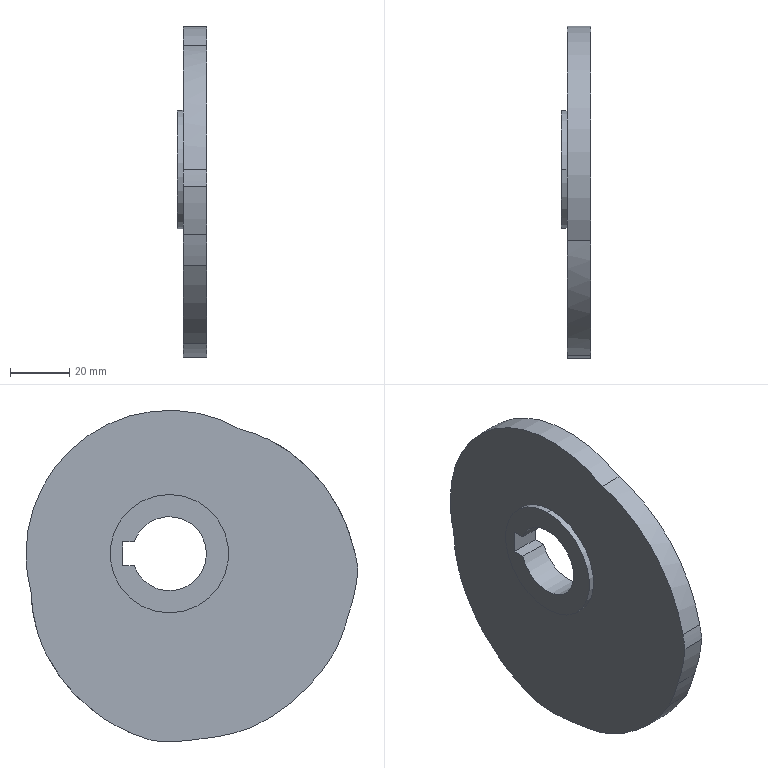Part | NX | 1 solid | 20 faces | box 10 x 112.057 x 111.8 mm | volume 75141 mm3 | cylinder 12 | plane 6 | spline 2 | commonest cylinder face diameters 25 x2 40 x2 96.8 x2 124.139 x1 126.8 x1 127.634 x1
STEP:
#1=CARTESIAN_POINT('',(-4.,46.751,-12.527));
#2=VERTEX_POINT('',#1);
#3=CARTESIAN_POINT('',(-4.,48.4,0.));
#4=VERTEX_POINT('',#3);
#5=CARTESIAN_POINT('',(-4.,0.,0.));
#6=DIRECTION('',(1.,0.,0.));
#7=DIRECTION('',(0.,1.,0.));
#8=AXIS2_PLACEMENT_3D('',#5,#6,#7);
#9=CIRCLE('',#8,48.4);
#10=EDGE_CURVE('',#2,#4,#9,.T.);
#11=ORIENTED_EDGE('',*,*,#10,.F.);
#12=CARTESIAN_POINT('',(-4.,5.526,-63.159));
#13=VERTEX_POINT('',#12);
#14=CARTESIAN_POINT('',(-4.,46.751,-12.527));
#15=CARTESIAN_POINT('',(-4.,46.716,-15.104));
#16=CARTESIAN_POINT('',(-4.,46.362,-18.915));
#17=CARTESIAN_POINT('',(-4.,45.21,-24.184));
#18=CARTESIAN_POINT('',(-4.,44.045,-28.007));
#19=CARTESIAN_POINT('',(-4.,42.505,-31.909));
#20=CARTESIAN_POINT('',(-4.,40.684,-35.618));
#21=CARTESIAN_POINT('',(-4.,38.469,-39.345));
#22=CARTESIAN_POINT('',(-4.,35.998,-42.831));
#23=CARTESIAN_POINT('',(-4.,33.129,-46.264));
#24=CARTESIAN_POINT('',(-4.,30.037,-49.413));
#25=CARTESIAN_POINT('',(-4.,26.555,-52.439));
#26=CARTESIAN_POINT('',(-4.,22.888,-55.142));
#27=CARTESIAN_POINT('',(-4.,18.854,-57.651));
#28=CARTESIAN_POINT('',(-4.,13.277,-60.529));
#29=CARTESIAN_POINT('',(-4.,8.665,-62.261));
#30=CARTESIAN_POINT('',(-4.,5.526,-63.159));
#31=B_SPLINE_CURVE_WITH_KNOTS('',3,(#14,#15,#16,#17,#18,#19,#20,#21,#22,#23,#24,#25,#26,#27,#28,#29,#30),.UNSPECIFIED.,.F.,.F.,(4,1,1,1,1,1,1,1,1,1,1,1,1,1,4),(0.00000001,0.125,0.1875,0.25,0.3125,0.375,0.4375,0.5,0.5625,0.625,0.6875,0.75,0.8125,0.875,1.),.UNSPECIFIED.);
#32=EDGE_CURVE('',#13,#2,#31,.F.);
#33=ORIENTED_EDGE('',*,*,#32,.F.);
#34=CARTESIAN_POINT('',(-4.,-11.009,-62.437));
#35=VERTEX_POINT('',#34);
#36=CARTESIAN_POINT('',(-4.,0.,0.));
#37=DIRECTION('',(1.,0.,0.));
#38=DIRECTION('',(0.,-0.1736,-0.9848));
#39=AXIS2_PLACEMENT_3D('',#36,#37,#38);
#40=CIRCLE('',#39,63.4);
#41=EDGE_CURVE('',#35,#13,#40,.T.);
#42=ORIENTED_EDGE('',*,*,#41,.F.);
#43=CARTESIAN_POINT('',(-4.,-27.428,-58.819));
#44=VERTEX_POINT('',#43);
#45=CARTESIAN_POINT('',(-4.,-5.606,1.151));
#46=DIRECTION('',(1.,0.,0.));
#47=DIRECTION('',(0.,-0.342,-0.9397));
#48=AXIS2_PLACEMENT_3D('',#45,#46,#47);
#49=CIRCLE('',#48,63.817);
#50=EDGE_CURVE('',#44,#35,#49,.T.);
#51=ORIENTED_EDGE('',*,*,#50,.F.);
#52=CARTESIAN_POINT('',(-4.,-56.205,-32.45));
#53=VERTEX_POINT('',#52);
#54=CARTESIAN_POINT('',(-4.,0.,0.));
#55=DIRECTION('',(1.,0.,0.));
#56=DIRECTION('',(0.,-0.866,-0.5));
#57=AXIS2_PLACEMENT_3D('',#54,#55,#56);
#58=CIRCLE('',#57,64.9);
#59=EDGE_CURVE('',#53,#44,#58,.T.);
#60=ORIENTED_EDGE('',*,*,#59,.F.);
#61=CARTESIAN_POINT('',(-4.,-60.047,-21.855));
#62=VERTEX_POINT('',#61);
#63=CARTESIAN_POINT('',(-4.,2.003,-5.352));
#64=DIRECTION('',(1.,0.,0.));
#65=DIRECTION('',(0.,-0.9664,-0.257));
#66=AXIS2_PLACEMENT_3D('',#63,#64,#65);
#67=CIRCLE('',#66,64.207);
#68=EDGE_CURVE('',#62,#53,#67,.T.);
#69=ORIENTED_EDGE('',*,*,#68,.F.);
#70=CARTESIAN_POINT('',(-4.,-63.657,-5.569));
#71=VERTEX_POINT('',#70);
#72=CARTESIAN_POINT('',(-4.,0.,0.));
#73=DIRECTION('',(1.,0.,0.));
#74=DIRECTION('',(0.,-0.9962,-0.08716));
#75=AXIS2_PLACEMENT_3D('',#72,#73,#74);
#76=CIRCLE('',#75,63.9);
#77=EDGE_CURVE('',#71,#62,#76,.T.);
#78=ORIENTED_EDGE('',*,*,#77,.F.);
#79=CARTESIAN_POINT('',(-4.,-62.708,0.000004523));
#80=VERTEX_POINT('',#79);
#81=CARTESIAN_POINT('',(-4.,-2.058,-13.201));
#82=DIRECTION('',(1.,0.,0.));
#83=DIRECTION('',(0.,-0.9771,0.2127));
#84=AXIS2_PLACEMENT_3D('',#81,#82,#83);
#85=CIRCLE('',#84,62.069);
#86=EDGE_CURVE('',#80,#71,#85,.T.);
#87=ORIENTED_EDGE('',*,*,#86,.F.);
#88=CARTESIAN_POINT('',(-4.,-24.2,41.916));
#89=VERTEX_POINT('',#88);
#90=CARTESIAN_POINT('',(-4.,-62.708,0.00001413));
#91=CARTESIAN_POINT('',(-4.,-61.523,5.434));
#92=CARTESIAN_POINT('',(-4.,-57.687,15.802));
#93=CARTESIAN_POINT('',(-4.,-48.504,28.366));
#94=CARTESIAN_POINT('',(-4.,-38.885,35.892));
#95=CARTESIAN_POINT('',(-4.,-30.566,39.982));
#96=CARTESIAN_POINT('',(-4.,-26.354,41.369));
#97=CARTESIAN_POINT('',(-4.,-24.2,41.916));
#98=B_SPLINE_CURVE_WITH_KNOTS('',3,(#90,#91,#92,#93,#94,#95,#96,#97),.UNSPECIFIED.,.F.,.F.,(4,1,1,1,1,4),(0.,0.25,0.5,0.75,0.875,1.),.UNSPECIFIED.);
#99=EDGE_CURVE('',#89,#80,#98,.F.);
#100=ORIENTED_EDGE('',*,*,#99,.F.);
#101=CARTESIAN_POINT('',(-4.,0.,0.));
#102=DIRECTION('',(1.,0.,0.));
#103=DIRECTION('',(0.,1.,0.));
#104=AXIS2_PLACEMENT_3D('',#101,#102,#103);
#105=CIRCLE('',#104,48.4);
#106=EDGE_CURVE('',#4,#89,#105,.T.);
#107=ORIENTED_EDGE('',*,*,#106,.F.);
#108=EDGE_LOOP('',(#11,#33,#42,#51,#60,#69,#78,#87,#100,#107));
#109=FACE_BOUND('',#108,.T.);
#110=CARTESIAN_POINT('',(-4.,0.,20.));
#111=VERTEX_POINT('',#110);
#112=CARTESIAN_POINT('',(-4.,0.,-20.));
#113=VERTEX_POINT('',#112);
#114=CARTESIAN_POINT('',(-4.,0.,0.));
#115=DIRECTION('',(-1.,0.,0.));
#116=DIRECTION('',(0.,0.,1.));
#117=AXIS2_PLACEMENT_3D('',#114,#115,#116);
#118=CIRCLE('',#117,20.);
#119=EDGE_CURVE('',#111,#113,#118,.T.);
#120=ORIENTED_EDGE('',*,*,#119,.F.);
#121=CARTESIAN_POINT('',(-4.,0.,0.));
#122=DIRECTION('',(-1.,0.,0.));
#123=DIRECTION('',(0.,0.,1.));
#124=AXIS2_PLACEMENT_3D('',#121,#122,#123);
#125=CIRCLE('',#124,20.);
#126=EDGE_CURVE('',#113,#111,#125,.T.);
#127=ORIENTED_EDGE('',*,*,#126,.F.);
#128=EDGE_LOOP('',(#120,#127));
#129=FACE_BOUND('',#128,.T.);
#130=CARTESIAN_POINT('',(-4.,0.,0.));
#131=DIRECTION('',(1.,0.,0.));
#132=DIRECTION('',(0.,1.,0.));
#133=AXIS2_PLACEMENT_3D('',#130,#131,#132);
#134=PLANE('',#133);
#135=ADVANCED_FACE('',(#109,#129),#134,.F.);
#136=CARTESIAN_POINT('',(4.,48.4,0.));
#137=VERTEX_POINT('',#136);
#138=CARTESIAN_POINT('',(-4.,48.4,0.));
#139=DIRECTION('',(1.,0.,0.));
#140=VECTOR('',#139,1000.);
#141=LINE('',#138,#140);
#142=EDGE_CURVE('',#4,#137,#141,.T.);
#143=ORIENTED_EDGE('',*,*,#142,.F.);
#144=ORIENTED_EDGE('',*,*,#106,.T.);
#145=CARTESIAN_POINT('',(4.,-24.2,41.916));
#146=VERTEX_POINT('',#145);
#147=CARTESIAN_POINT('',(-4.,-24.2,41.916));
#148=CARTESIAN_POINT('',(-1.333,-24.2,41.916));
#149=CARTESIAN_POINT('',(1.333,-24.2,41.916));
#150=CARTESIAN_POINT('',(4.,-24.2,41.916));
#151=B_SPLINE_CURVE_WITH_KNOTS('',3,(#147,#148,#149,#150),.UNSPECIFIED.,.F.,.F.,(4,4),(0.,1.),.UNSPECIFIED.);
#152=EDGE_CURVE('',#89,#146,#151,.T.);
#153=ORIENTED_EDGE('',*,*,#152,.T.);
#154=CARTESIAN_POINT('',(4.,0.,0.));
#155=DIRECTION('',(-1.,0.,0.));
#156=DIRECTION('',(0.,-0.5,0.866));
#157=AXIS2_PLACEMENT_3D('',#154,#155,#156);
#158=CIRCLE('',#157,48.4);
#159=EDGE_CURVE('',#146,#137,#158,.T.);
#160=ORIENTED_EDGE('',*,*,#159,.T.);
#161=EDGE_LOOP('',(#143,#144,#153,#160));
#162=FACE_BOUND('',#161,.T.);
#163=CARTESIAN_POINT('',(-4.,0.,0.));
#164=DIRECTION('',(1.,0.,0.));
#165=DIRECTION('',(0.,1.,0.));
#166=AXIS2_PLACEMENT_3D('',#163,#164,#165);
#167=CYLINDRICAL_SURFACE('',#166,48.4);
#168=ADVANCED_FACE('',(#162),#167,.T.);
#169=CARTESIAN_POINT('',(4.,5.526,-63.159));
#170=VERTEX_POINT('',#169);
#171=CARTESIAN_POINT('',(-4.,5.526,-63.159));
#172=CARTESIAN_POINT('',(-1.333,5.526,-63.159));
#173=CARTESIAN_POINT('',(1.333,5.526,-63.159));
#174=CARTESIAN_POINT('',(4.,5.526,-63.159));
#175=B_SPLINE_CURVE_WITH_KNOTS('',3,(#171,#172,#173,#174),.UNSPECIFIED.,.F.,.F.,(4,4),(0.,1.),.UNSPECIFIED.);
#176=EDGE_CURVE('',#13,#170,#175,.T.);
#177=ORIENTED_EDGE('',*,*,#176,.F.);
#178=ORIENTED_EDGE('',*,*,#32,.T.);
#179=CARTESIAN_POINT('',(4.,46.751,-12.527));
#180=VERTEX_POINT('',#179);
#181=CARTESIAN_POINT('',(4.,46.751,-12.527));
#182=CARTESIAN_POINT('',(1.333,46.751,-12.527));
#183=CARTESIAN_POINT('',(-1.333,46.751,-12.527));
#184=CARTESIAN_POINT('',(-4.,46.751,-12.527));
#185=B_SPLINE_CURVE_WITH_KNOTS('',3,(#181,#182,#183,#184),.UNSPECIFIED.,.F.,.F.,(4,4),(0.,1.),.UNSPECIFIED.);
#186=EDGE_CURVE('',#180,#2,#185,.T.);
#187=ORIENTED_EDGE('',*,*,#186,.F.);
#188=CARTESIAN_POINT('',(4.,5.526,-63.159));
#189=CARTESIAN_POINT('',(4.,8.665,-62.261));
#190=CARTESIAN_POINT('',(4.,13.278,-60.528));
#191=CARTESIAN_POINT('',(4.,18.853,-57.651));
#192=CARTESIAN_POINT('',(4.,22.889,-55.141));
#193=CARTESIAN_POINT('',(4.,26.554,-52.439));
#194=CARTESIAN_POINT('',(4.,30.038,-49.413));
#195=CARTESIAN_POINT('',(4.,33.129,-46.265));
#196=CARTESIAN_POINT('',(4.,35.998,-42.83));
#197=CARTESIAN_POINT('',(4.,38.468,-39.346));
#198=CARTESIAN_POINT('',(4.,40.684,-35.618));
#199=CARTESIAN_POINT('',(4.,42.505,-31.91));
#200=CARTESIAN_POINT('',(4.,44.046,-28.006));
#201=CARTESIAN_POINT('',(4.,45.21,-24.185));
#202=CARTESIAN_POINT('',(4.,46.362,-18.914));
#203=CARTESIAN_POINT('',(4.,46.716,-15.104));
#204=CARTESIAN_POINT('',(4.,46.751,-12.527));
#205=B_SPLINE_CURVE_WITH_KNOTS('',3,(#188,#189,#190,#191,#192,#193,#194,#195,#196,#197,#198,#199,#200,#201,#202,#203,#204),.UNSPECIFIED.,.F.,.F.,(4,1,1,1,1,1,1,1,1,1,1,1,1,1,4),(0.,0.125,0.1875,0.25,0.3125,0.375,0.4375,0.5,0.5625,0.625,0.6875,0.75,0.8125,0.875,1.),.UNSPECIFIED.);
#206=EDGE_CURVE('',#180,#170,#205,.F.);
#207=ORIENTED_EDGE('',*,*,#206,.T.);
#208=EDGE_LOOP('',(#177,#178,#187,#207));
#209=FACE_BOUND('',#208,.T.);
#210=CARTESIAN_POINT('',(4.,5.526,-63.159));
#211=CARTESIAN_POINT('',(-4.,5.526,-63.159));
#212=CARTESIAN_POINT('',(4.,11.847,-61.351));
#213=CARTESIAN_POINT('',(-4.,11.847,-61.351));
#214=CARTESIAN_POINT('',(4.,23.543,-55.825));
#215=CARTESIAN_POINT('',(-4.,23.543,-55.825));
#216=CARTESIAN_POINT('',(4.,36.792,-43.244));
#217=CARTESIAN_POINT('',(-4.,36.792,-43.244));
#218=CARTESIAN_POINT('',(4.,44.88,-28.132));
#219=CARTESIAN_POINT('',(-4.,44.88,-28.132));
#220=CARTESIAN_POINT('',(4.,46.683,-17.61));
#221=CARTESIAN_POINT('',(-4.,46.683,-17.61));
#222=CARTESIAN_POINT('',(4.,46.751,-12.527));
#223=CARTESIAN_POINT('',(-4.,46.751,-12.527));
#224=B_SPLINE_SURFACE_WITH_KNOTS('',3,1,((#210,#211),(#212,#213),(#214,#215),(#216,#217),(#218,#219),(#220,#221),(#222,#223)),.SURF_OF_LINEAR_EXTRUSION.,.F.,.F.,.F.,(4,1,1,1,4),(2,2),(0.008679,0.2537,0.4987,0.7438,0.9888),(0.,1.),.UNSPECIFIED.);
#225=ADVANCED_FACE('',(#209),#224,.F.);
#226=CARTESIAN_POINT('',(4.,-11.009,-62.437));
#227=VERTEX_POINT('',#226);
#228=CARTESIAN_POINT('',(4.,-11.009,-62.437));
#229=CARTESIAN_POINT('',(1.333,-11.009,-62.437));
#230=CARTESIAN_POINT('',(-1.333,-11.009,-62.437));
#231=CARTESIAN_POINT('',(-4.,-11.009,-62.437));
#232=B_SPLINE_CURVE_WITH_KNOTS('',3,(#228,#229,#230,#231),.UNSPECIFIED.,.F.,.F.,(4,4),(0.,1.),.UNSPECIFIED.);
#233=EDGE_CURVE('',#35,#227,#232,.F.);
#234=ORIENTED_EDGE('',*,*,#233,.F.);
#235=ORIENTED_EDGE('',*,*,#41,.T.);
#236=ORIENTED_EDGE('',*,*,#176,.T.);
#237=CARTESIAN_POINT('',(4.,0.,0.));
#238=DIRECTION('',(-1.,0.,0.));
#239=DIRECTION('',(0.,0.08716,-0.9962));
#240=AXIS2_PLACEMENT_3D('',#237,#238,#239);
#241=CIRCLE('',#240,63.4);
#242=EDGE_CURVE('',#170,#227,#241,.T.);
#243=ORIENTED_EDGE('',*,*,#242,.T.);
#244=EDGE_LOOP('',(#234,#235,#236,#243));
#245=FACE_BOUND('',#244,.T.);
#246=CARTESIAN_POINT('',(-4.,0.,0.));
#247=DIRECTION('',(1.,0.,0.));
#248=DIRECTION('',(0.,-0.1736,-0.9848));
#249=AXIS2_PLACEMENT_3D('',#246,#247,#248);
#250=CYLINDRICAL_SURFACE('',#249,63.4);
#251=ADVANCED_FACE('',(#245),#250,.T.);
#252=CARTESIAN_POINT('',(4.,-27.428,-58.819));
#253=VERTEX_POINT('',#252);
#254=CARTESIAN_POINT('',(4.,-27.428,-58.819));
#255=CARTESIAN_POINT('',(1.333,-27.428,-58.819));
#256=CARTESIAN_POINT('',(-1.333,-27.428,-58.819));
#257=CARTESIAN_POINT('',(-4.,-27.428,-58.819));
#258=B_SPLINE_CURVE_WITH_KNOTS('',3,(#254,#255,#256,#257),.UNSPECIFIED.,.F.,.F.,(4,4),(0.,1.),.UNSPECIFIED.);
#259=EDGE_CURVE('',#253,#44,#258,.T.);
#260=ORIENTED_EDGE('',*,*,#259,.T.);
#261=ORIENTED_EDGE('',*,*,#50,.T.);
#262=ORIENTED_EDGE('',*,*,#233,.T.);
#263=CARTESIAN_POINT('',(4.,-5.606,1.151));
#264=DIRECTION('',(-1.,0.,0.));
#265=DIRECTION('',(0.,-0.08467,-0.9964));
#266=AXIS2_PLACEMENT_3D('',#263,#264,#265);
#267=CIRCLE('',#266,63.817);
#268=EDGE_CURVE('',#227,#253,#267,.T.);
#269=ORIENTED_EDGE('',*,*,#268,.T.);
#270=EDGE_LOOP('',(#260,#261,#262,#269));
#271=FACE_BOUND('',#270,.T.);
#272=CARTESIAN_POINT('',(0.,-5.606,1.151));
#273=DIRECTION('',(-1.,0.,0.));
#274=DIRECTION('',(0.,-0.3419,-0.9397));
#275=AXIS2_PLACEMENT_3D('',#272,#273,#274);
#276=CYLINDRICAL_SURFACE('',#275,63.817);
#277=ADVANCED_FACE('',(#271),#276,.T.);
#278=CARTESIAN_POINT('',(4.,-56.205,-32.45));
#279=VERTEX_POINT('',#278);
#280=CARTESIAN_POINT('',(4.,-56.205,-32.45));
#281=CARTESIAN_POINT('',(1.333,-56.205,-32.45));
#282=CARTESIAN_POINT('',(-1.333,-56.205,-32.45));
#283=CARTESIAN_POINT('',(-4.,-56.205,-32.45));
#284=B_SPLINE_CURVE_WITH_KNOTS('',3,(#280,#281,#282,#283),.UNSPECIFIED.,.F.,.F.,(4,4),(0.,1.),.UNSPECIFIED.);
#285=EDGE_CURVE('',#53,#279,#284,.F.);
#286=ORIENTED_EDGE('',*,*,#285,.F.);
#287=ORIENTED_EDGE('',*,*,#59,.T.);
#288=ORIENTED_EDGE('',*,*,#259,.F.);
#289=CARTESIAN_POINT('',(4.,0.,0.));
#290=DIRECTION('',(-1.,0.,0.));
#291=DIRECTION('',(0.,-0.4227,-0.9063));
#292=AXIS2_PLACEMENT_3D('',#289,#290,#291);
#293=CIRCLE('',#292,64.9);
#294=EDGE_CURVE('',#253,#279,#293,.T.);
#295=ORIENTED_EDGE('',*,*,#294,.T.);
#296=EDGE_LOOP('',(#286,#287,#288,#295));
#297=FACE_BOUND('',#296,.T.);
#298=CARTESIAN_POINT('',(-4.,0.,0.));
#299=DIRECTION('',(1.,0.,0.));
#300=DIRECTION('',(0.,-0.866,-0.5));
#301=AXIS2_PLACEMENT_3D('',#298,#299,#300);
#302=CYLINDRICAL_SURFACE('',#301,64.9);
#303=ADVANCED_FACE('',(#297),#302,.T.);
#304=CARTESIAN_POINT('',(4.,-60.047,-21.855));
#305=VERTEX_POINT('',#304);
#306=CARTESIAN_POINT('',(4.,-60.047,-21.855));
#307=CARTESIAN_POINT('',(1.333,-60.047,-21.855));
#308=CARTESIAN_POINT('',(-1.333,-60.047,-21.855));
#309=CARTESIAN_POINT('',(-4.,-60.047,-21.855));
#310=B_SPLINE_CURVE_WITH_KNOTS('',3,(#306,#307,#308,#309),.UNSPECIFIED.,.F.,.F.,(4,4),(0.,1.),.UNSPECIFIED.);
#311=EDGE_CURVE('',#305,#62,#310,.T.);
#312=ORIENTED_EDGE('',*,*,#311,.T.);
#313=ORIENTED_EDGE('',*,*,#68,.T.);
#314=ORIENTED_EDGE('',*,*,#285,.T.);
#315=CARTESIAN_POINT('',(4.,2.003,-5.352));
#316=DIRECTION('',(-1.,0.,0.));
#317=DIRECTION('',(0.,-0.9066,-0.422));
#318=AXIS2_PLACEMENT_3D('',#315,#316,#317);
#319=CIRCLE('',#318,64.207);
#320=EDGE_CURVE('',#279,#305,#319,.T.);
#321=ORIENTED_EDGE('',*,*,#320,.T.);
#322=EDGE_LOOP('',(#312,#313,#314,#321));
#323=FACE_BOUND('',#322,.T.);
#324=CARTESIAN_POINT('',(0.,2.003,-5.352));
#325=DIRECTION('',(-1.,0.,0.));
#326=DIRECTION('',(0.,-0.9664,-0.257));
#327=AXIS2_PLACEMENT_3D('',#324,#325,#326);
#328=CYLINDRICAL_SURFACE('',#327,64.207);
#329=ADVANCED_FACE('',(#323),#328,.T.);
#330=CARTESIAN_POINT('',(4.,-63.657,-5.569));
#331=VERTEX_POINT('',#330);
#332=CARTESIAN_POINT('',(4.,-63.657,-5.569));
#333=CARTESIAN_POINT('',(1.333,-63.657,-5.569));
#334=CARTESIAN_POINT('',(-1.333,-63.657,-5.569));
#335=CARTESIAN_POINT('',(-4.,-63.657,-5.569));
#336=B_SPLINE_CURVE_WITH_KNOTS('',3,(#332,#333,#334,#335),.UNSPECIFIED.,.F.,.F.,(4,4),(0.,1.),.UNSPECIFIED.);
#337=EDGE_CURVE('',#71,#331,#336,.F.);
#338=ORIENTED_EDGE('',*,*,#337,.F.);
#339=ORIENTED_EDGE('',*,*,#77,.T.);
#340=ORIENTED_EDGE('',*,*,#311,.F.);
#341=CARTESIAN_POINT('',(4.,0.,0.));
#342=DIRECTION('',(-1.,0.,0.));
#343=DIRECTION('',(0.,-0.9397,-0.342));
#344=AXIS2_PLACEMENT_3D('',#341,#342,#343);
#345=CIRCLE('',#344,63.9);
#346=EDGE_CURVE('',#305,#331,#345,.T.);
#347=ORIENTED_EDGE('',*,*,#346,.T.);
#348=EDGE_LOOP('',(#338,#339,#340,#347));
#349=FACE_BOUND('',#348,.T.);
#350=CARTESIAN_POINT('',(-4.,0.,0.));
#351=DIRECTION('',(1.,0.,0.));
#352=DIRECTION('',(0.,-0.9962,-0.08716));
#353=AXIS2_PLACEMENT_3D('',#350,#351,#352);
#354=CYLINDRICAL_SURFACE('',#353,63.9);
#355=ADVANCED_FACE('',(#349),#354,.T.);
#356=CARTESIAN_POINT('',(4.,-62.708,0.000004523));
#357=VERTEX_POINT('',#356);
#358=CARTESIAN_POINT('',(4.,-62.708,0.00001413));
#359=CARTESIAN_POINT('',(1.333,-62.708,0.00001413));
#360=CARTESIAN_POINT('',(-1.333,-62.708,0.00001413));
#361=CARTESIAN_POINT('',(-4.,-62.708,0.00001413));
#362=B_SPLINE_CURVE_WITH_KNOTS('',3,(#358,#359,#360,#361),.UNSPECIFIED.,.F.,.F.,(4,4),(0.,1.),.UNSPECIFIED.);
#363=EDGE_CURVE('',#357,#80,#362,.T.);
#364=ORIENTED_EDGE('',*,*,#363,.T.);
#365=ORIENTED_EDGE('',*,*,#86,.T.);
#366=ORIENTED_EDGE('',*,*,#337,.T.);
#367=CARTESIAN_POINT('',(4.,-2.058,-13.201));
#368=DIRECTION('',(-1.,0.,0.));
#369=DIRECTION('',(0.,-0.9924,0.123));
#370=AXIS2_PLACEMENT_3D('',#367,#368,#369);
#371=CIRCLE('',#370,62.069);
#372=EDGE_CURVE('',#331,#357,#371,.T.);
#373=ORIENTED_EDGE('',*,*,#372,.T.);
#374=EDGE_LOOP('',(#364,#365,#366,#373));
#375=FACE_BOUND('',#374,.T.);
#376=CARTESIAN_POINT('',(0.,-2.058,-13.201));
#377=DIRECTION('',(-1.,0.,0.));
#378=DIRECTION('',(0.,-0.9771,0.2127));
#379=AXIS2_PLACEMENT_3D('',#376,#377,#378);
#380=CYLINDRICAL_SURFACE('',#379,62.069);
#381=ADVANCED_FACE('',(#375),#380,.T.);
#382=ORIENTED_EDGE('',*,*,#152,.F.);
#383=ORIENTED_EDGE('',*,*,#99,.T.);
#384=ORIENTED_EDGE('',*,*,#363,.F.);
#385=CARTESIAN_POINT('',(4.,-24.2,41.916));
#386=CARTESIAN_POINT('',(4.,-26.354,41.369));
#387=CARTESIAN_POINT('',(4.,-30.566,39.981));
#388=CARTESIAN_POINT('',(4.,-38.885,35.892));
#389=CARTESIAN_POINT('',(4.,-48.504,28.366));
#390=CARTESIAN_POINT('',(4.,-57.688,15.802));
#391=CARTESIAN_POINT('',(4.,-61.523,5.435));
#392=CARTESIAN_POINT('',(4.,-62.708,0.00001413));
#393=B_SPLINE_CURVE_WITH_KNOTS('',3,(#385,#386,#387,#388,#389,#390,#391,#392),.UNSPECIFIED.,.F.,.F.,(4,1,1,1,1,4),(0.000000006,0.125,0.25,0.5,0.75,1.),.UNSPECIFIED.);
#394=EDGE_CURVE('',#357,#146,#393,.F.);
#395=ORIENTED_EDGE('',*,*,#394,.T.);
#396=EDGE_LOOP('',(#382,#383,#384,#395));
#397=FACE_BOUND('',#396,.T.);
#398=CARTESIAN_POINT('',(4.,-24.2,41.916));
#399=CARTESIAN_POINT('',(-4.,-24.2,41.916));
#400=CARTESIAN_POINT('',(4.,-32.708,39.757));
#401=CARTESIAN_POINT('',(-4.,-32.708,39.757));
#402=CARTESIAN_POINT('',(4.,-49.707,30.203));
#403=CARTESIAN_POINT('',(-4.,-49.707,30.203));
#404=CARTESIAN_POINT('',(4.,-60.323,10.944));
#405=CARTESIAN_POINT('',(-4.,-60.323,10.944));
#406=CARTESIAN_POINT('',(4.,-62.708,-0.000005119));
#407=CARTESIAN_POINT('',(-4.,-62.708,-0.000005119));
#408=B_SPLINE_SURFACE_WITH_KNOTS('',3,1,((#398,#399),(#400,#401),(#402,#403),(#404,#405),(#406,#407)),.SURF_OF_LINEAR_EXTRUSION.,.F.,.F.,.F.,(4,1,4),(2,2),(0.01117,0.5012,0.9913),(0.,1.),.UNSPECIFIED.);
#409=ADVANCED_FACE('',(#397),#408,.F.);
#410=ORIENTED_EDGE('',*,*,#159,.F.);
#411=ORIENTED_EDGE('',*,*,#394,.F.);
#412=ORIENTED_EDGE('',*,*,#372,.F.);
#413=ORIENTED_EDGE('',*,*,#346,.F.);
#414=ORIENTED_EDGE('',*,*,#320,.F.);
#415=ORIENTED_EDGE('',*,*,#294,.F.);
#416=ORIENTED_EDGE('',*,*,#268,.F.);
#417=ORIENTED_EDGE('',*,*,#242,.F.);
#418=ORIENTED_EDGE('',*,*,#206,.F.);
#419=CARTESIAN_POINT('',(4.,0.,0.));
#420=DIRECTION('',(-1.,0.,0.));
#421=DIRECTION('',(0.,-0.5,0.866));
#422=AXIS2_PLACEMENT_3D('',#419,#420,#421);
#423=CIRCLE('',#422,48.4);
#424=EDGE_CURVE('',#137,#180,#423,.T.);
#425=ORIENTED_EDGE('',*,*,#424,.F.);
#426=EDGE_LOOP('',(#410,#411,#412,#413,#414,#415,#416,#417,#418,#425));
#427=FACE_BOUND('',#426,.T.);
#428=CARTESIAN_POINT('',(4.,11.843,4.));
#429=VERTEX_POINT('',#428);
#430=CARTESIAN_POINT('',(4.,-12.5,0.));
#431=VERTEX_POINT('',#430);
#432=CARTESIAN_POINT('',(4.,0.,0.));
#433=DIRECTION('',(1.,0.,0.));
#434=DIRECTION('',(0.,-1.,0.));
#435=AXIS2_PLACEMENT_3D('',#432,#433,#434);
#436=CIRCLE('',#435,12.5);
#437=EDGE_CURVE('',#429,#431,#436,.T.);
#438=ORIENTED_EDGE('',*,*,#437,.F.);
#439=CARTESIAN_POINT('',(4.,15.8,4.));
#440=VERTEX_POINT('',#439);
#441=CARTESIAN_POINT('',(4.,11.843,4.));
#442=DIRECTION('',(0.,1.,0.));
#443=VECTOR('',#442,1000.);
#444=LINE('',#441,#443);
#445=EDGE_CURVE('',#429,#440,#444,.T.);
#446=ORIENTED_EDGE('',*,*,#445,.T.);
#447=CARTESIAN_POINT('',(4.,15.8,-4.));
#448=VERTEX_POINT('',#447);
#449=CARTESIAN_POINT('',(4.,15.8,4.));
#450=DIRECTION('',(0.,0.,-1.));
#451=VECTOR('',#450,1000.);
#452=LINE('',#449,#451);
#453=EDGE_CURVE('',#440,#448,#452,.T.);
#454=ORIENTED_EDGE('',*,*,#453,.T.);
#455=CARTESIAN_POINT('',(4.,11.843,-4.));
#456=VERTEX_POINT('',#455);
#457=CARTESIAN_POINT('',(4.,15.8,-4.));
#458=DIRECTION('',(0.,-1.,0.));
#459=VECTOR('',#458,1000.);
#460=LINE('',#457,#459);
#461=EDGE_CURVE('',#448,#456,#460,.T.);
#462=ORIENTED_EDGE('',*,*,#461,.T.);
#463=CARTESIAN_POINT('',(4.,0.,0.));
#464=DIRECTION('',(1.,0.,0.));
#465=DIRECTION('',(0.,-1.,0.));
#466=AXIS2_PLACEMENT_3D('',#463,#464,#465);
#467=CIRCLE('',#466,12.5);
#468=EDGE_CURVE('',#431,#456,#467,.T.);
#469=ORIENTED_EDGE('',*,*,#468,.F.);
#470=EDGE_LOOP('',(#438,#446,#454,#462,#469));
#471=FACE_BOUND('',#470,.T.);
#472=CARTESIAN_POINT('',(4.,0.,0.));
#473=DIRECTION('',(1.,0.,0.));
#474=DIRECTION('',(0.,1.,0.));
#475=AXIS2_PLACEMENT_3D('',#472,#473,#474);
#476=PLANE('',#475);
#477=ADVANCED_FACE('',(#427,#471),#476,.T.);
#478=CARTESIAN_POINT('',(-6.,-12.5,0.));
#479=VERTEX_POINT('',#478);
#480=CARTESIAN_POINT('',(-4.4,-12.5,0.));
#481=DIRECTION('',(1.,0.,0.));
#482=VECTOR('',#481,1000.);
#483=LINE('',#480,#482);
#484=EDGE_CURVE('',#479,#431,#483,.T.);
#485=ORIENTED_EDGE('',*,*,#484,.F.);
#486=CARTESIAN_POINT('',(-6.,11.843,4.));
#487=VERTEX_POINT('',#486);
#488=CARTESIAN_POINT('',(-6.,0.,0.));
#489=DIRECTION('',(-1.,0.,0.));
#490=DIRECTION('',(0.,0.9474,-0.32));
#491=AXIS2_PLACEMENT_3D('',#488,#489,#490);
#492=CIRCLE('',#491,12.5);
#493=EDGE_CURVE('',#479,#487,#492,.T.);
#494=ORIENTED_EDGE('',*,*,#493,.T.);
#495=CARTESIAN_POINT('',(4.,11.843,4.));
#496=DIRECTION('',(-1.,0.,0.));
#497=VECTOR('',#496,1000.);
#498=LINE('',#495,#497);
#499=EDGE_CURVE('',#429,#487,#498,.T.);
#500=ORIENTED_EDGE('',*,*,#499,.F.);
#501=ORIENTED_EDGE('',*,*,#437,.T.);
#502=EDGE_LOOP('',(#485,#494,#500,#501));
#503=FACE_BOUND('',#502,.T.);
#504=CARTESIAN_POINT('',(-4.4,0.,0.));
#505=DIRECTION('',(1.,0.,0.));
#506=DIRECTION('',(0.,-1.,0.));
#507=AXIS2_PLACEMENT_3D('',#504,#505,#506);
#508=CYLINDRICAL_SURFACE('',#507,12.5);
#509=ADVANCED_FACE('',(#503),#508,.F.);
#510=CARTESIAN_POINT('',(-6.,15.8,4.));
#511=VERTEX_POINT('',#510);
#512=CARTESIAN_POINT('',(-6.,15.8,4.));
#513=DIRECTION('',(1.,0.,0.));
#514=VECTOR('',#513,1000.);
#515=LINE('',#512,#514);
#516=EDGE_CURVE('',#511,#440,#515,.T.);
#517=ORIENTED_EDGE('',*,*,#516,.T.);
#518=ORIENTED_EDGE('',*,*,#445,.F.);
#519=ORIENTED_EDGE('',*,*,#499,.T.);
#520=CARTESIAN_POINT('',(-6.,11.843,4.));
#521=DIRECTION('',(0.,1.,0.));
#522=VECTOR('',#521,1000.);
#523=LINE('',#520,#522);
#524=EDGE_CURVE('',#487,#511,#523,.T.);
#525=ORIENTED_EDGE('',*,*,#524,.T.);
#526=EDGE_LOOP('',(#517,#518,#519,#525));
#527=FACE_BOUND('',#526,.T.);
#528=CARTESIAN_POINT('',(4.,15.8,4.));
#529=DIRECTION('',(0.,0.,1.));
#530=DIRECTION('',(1.,0.,0.));
#531=AXIS2_PLACEMENT_3D('',#528,#529,#530);
#532=PLANE('',#531);
#533=ADVANCED_FACE('',(#527),#532,.F.);
#534=CARTESIAN_POINT('',(-6.,15.8,-4.));
#535=VERTEX_POINT('',#534);
#536=CARTESIAN_POINT('',(-6.,15.8,-4.));
#537=DIRECTION('',(1.,0.,0.));
#538=VECTOR('',#537,1000.);
#539=LINE('',#536,#538);
#540=EDGE_CURVE('',#535,#448,#539,.T.);
#541=ORIENTED_EDGE('',*,*,#540,.T.);
#542=ORIENTED_EDGE('',*,*,#453,.F.);
#543=ORIENTED_EDGE('',*,*,#516,.F.);
#544=CARTESIAN_POINT('',(-6.,15.8,4.));
#545=DIRECTION('',(0.,0.,-1.));
#546=VECTOR('',#545,1000.);
#547=LINE('',#544,#546);
#548=EDGE_CURVE('',#511,#535,#547,.T.);
#549=ORIENTED_EDGE('',*,*,#548,.T.);
#550=EDGE_LOOP('',(#541,#542,#543,#549));
#551=FACE_BOUND('',#550,.T.);
#552=CARTESIAN_POINT('',(4.,15.8,-4.));
#553=DIRECTION('',(0.,1.,0.));
#554=DIRECTION('',(1.,0.,0.));
#555=AXIS2_PLACEMENT_3D('',#552,#553,#554);
#556=PLANE('',#555);
#557=ADVANCED_FACE('',(#551),#556,.F.);
#558=CARTESIAN_POINT('',(-6.,11.843,-4.));
#559=VERTEX_POINT('',#558);
#560=CARTESIAN_POINT('',(-6.,11.843,-4.));
#561=DIRECTION('',(1.,0.,0.));
#562=VECTOR('',#561,1000.);
#563=LINE('',#560,#562);
#564=EDGE_CURVE('',#559,#456,#563,.T.);
#565=ORIENTED_EDGE('',*,*,#564,.T.);
#566=ORIENTED_EDGE('',*,*,#461,.F.);
#567=ORIENTED_EDGE('',*,*,#540,.F.);
#568=CARTESIAN_POINT('',(-6.,15.8,-4.));
#569=DIRECTION('',(0.,-1.,0.));
#570=VECTOR('',#569,1000.);
#571=LINE('',#568,#570);
#572=EDGE_CURVE('',#535,#559,#571,.T.);
#573=ORIENTED_EDGE('',*,*,#572,.T.);
#574=EDGE_LOOP('',(#565,#566,#567,#573));
#575=FACE_BOUND('',#574,.T.);
#576=CARTESIAN_POINT('',(4.,11.843,-4.));
#577=DIRECTION('',(0.,0.,-1.));
#578=DIRECTION('',(0.,-1.,0.));
#579=AXIS2_PLACEMENT_3D('',#576,#577,#578);
#580=PLANE('',#579);
#581=ADVANCED_FACE('',(#575),#580,.F.);
#582=CARTESIAN_POINT('',(-6.,0.,-20.));
#583=VERTEX_POINT('',#582);
#584=CARTESIAN_POINT('',(-6.,0.,20.));
#585=VERTEX_POINT('',#584);
#586=CARTESIAN_POINT('',(-6.,0.,0.));
#587=DIRECTION('',(1.,0.,0.));
#588=DIRECTION('',(0.,0.,-1.));
#589=AXIS2_PLACEMENT_3D('',#586,#587,#588);
#590=CIRCLE('',#589,20.);
#591=EDGE_CURVE('',#583,#585,#590,.T.);
#592=ORIENTED_EDGE('',*,*,#591,.F.);
#593=CARTESIAN_POINT('',(-6.,0.,0.));
#594=DIRECTION('',(1.,0.,0.));
#595=DIRECTION('',(0.,0.,-1.));
#596=AXIS2_PLACEMENT_3D('',#593,#594,#595);
#597=CIRCLE('',#596,20.);
#598=EDGE_CURVE('',#585,#583,#597,.T.);
#599=ORIENTED_EDGE('',*,*,#598,.F.);
#600=EDGE_LOOP('',(#592,#599));
#601=FACE_BOUND('',#600,.T.);
#602=CARTESIAN_POINT('',(-6.,0.,0.));
#603=DIRECTION('',(-1.,0.,0.));
#604=DIRECTION('',(0.,0.9474,-0.32));
#605=AXIS2_PLACEMENT_3D('',#602,#603,#604);
#606=CIRCLE('',#605,12.5);
#607=EDGE_CURVE('',#559,#479,#606,.T.);
#608=ORIENTED_EDGE('',*,*,#607,.F.);
#609=ORIENTED_EDGE('',*,*,#572,.F.);
#610=ORIENTED_EDGE('',*,*,#548,.F.);
#611=ORIENTED_EDGE('',*,*,#524,.F.);
#612=ORIENTED_EDGE('',*,*,#493,.F.);
#613=EDGE_LOOP('',(#608,#609,#610,#611,#612));
#614=FACE_BOUND('',#613,.T.);
#615=CARTESIAN_POINT('',(-6.,0.,0.));
#616=DIRECTION('',(-1.,0.,0.));
#617=DIRECTION('',(0.,0.,1.));
#618=AXIS2_PLACEMENT_3D('',#615,#616,#617);
#619=PLANE('',#618);
#620=ADVANCED_FACE('',(#601,#614),#619,.T.);
#621=ORIENTED_EDGE('',*,*,#591,.T.);
#622=CARTESIAN_POINT('',(-4.,0.,20.));
#623=DIRECTION('',(-1.,0.,0.));
#624=VECTOR('',#623,1000.);
#625=LINE('',#622,#624);
#626=EDGE_CURVE('',#585,#111,#625,.F.);
#627=ORIENTED_EDGE('',*,*,#626,.T.);
#628=ORIENTED_EDGE('',*,*,#119,.T.);
#629=CARTESIAN_POINT('',(-4.,0.,-20.));
#630=DIRECTION('',(-1.,0.,0.));
#631=VECTOR('',#630,1000.);
#632=LINE('',#629,#631);
#633=EDGE_CURVE('',#583,#113,#632,.F.);
#634=ORIENTED_EDGE('',*,*,#633,.F.);
#635=EDGE_LOOP('',(#621,#627,#628,#634));
#636=FACE_BOUND('',#635,.T.);
#637=CARTESIAN_POINT('',(-4.,0.,0.));
#638=DIRECTION('',(-1.,0.,0.));
#639=DIRECTION('',(0.,0.,-1.));
#640=AXIS2_PLACEMENT_3D('',#637,#638,#639);
#641=CYLINDRICAL_SURFACE('',#640,20.);
#642=ADVANCED_FACE('',(#636),#641,.T.);
#643=ORIENTED_EDGE('',*,*,#633,.T.);
#644=ORIENTED_EDGE('',*,*,#126,.T.);
#645=ORIENTED_EDGE('',*,*,#626,.F.);
#646=ORIENTED_EDGE('',*,*,#598,.T.);
#647=EDGE_LOOP('',(#643,#644,#645,#646));
#648=FACE_BOUND('',#647,.T.);
#649=CARTESIAN_POINT('',(-4.,0.,0.));
#650=DIRECTION('',(-1.,0.,0.));
#651=DIRECTION('',(0.,0.,-1.));
#652=AXIS2_PLACEMENT_3D('',#649,#650,#651);
#653=CYLINDRICAL_SURFACE('',#652,20.);
#654=ADVANCED_FACE('',(#648),#653,.T.);
#655=ORIENTED_EDGE('',*,*,#607,.T.);
#656=ORIENTED_EDGE('',*,*,#484,.T.);
#657=ORIENTED_EDGE('',*,*,#468,.T.);
#658=ORIENTED_EDGE('',*,*,#564,.F.);
#659=EDGE_LOOP('',(#655,#656,#657,#658));
#660=FACE_BOUND('',#659,.T.);
#661=CARTESIAN_POINT('',(-4.4,0.,0.));
#662=DIRECTION('',(1.,0.,0.));
#663=DIRECTION('',(0.,-1.,0.));
#664=AXIS2_PLACEMENT_3D('',#661,#662,#663);
#665=CYLINDRICAL_SURFACE('',#664,12.5);
#666=ADVANCED_FACE('',(#660),#665,.F.);
#667=ORIENTED_EDGE('',*,*,#10,.T.);
#668=ORIENTED_EDGE('',*,*,#142,.T.);
#669=ORIENTED_EDGE('',*,*,#424,.T.);
#670=ORIENTED_EDGE('',*,*,#186,.T.);
#671=EDGE_LOOP('',(#667,#668,#669,#670));
#672=FACE_BOUND('',#671,.T.);
#673=CARTESIAN_POINT('',(-4.,0.,0.));
#674=DIRECTION('',(1.,0.,0.));
#675=DIRECTION('',(0.,1.,0.));
#676=AXIS2_PLACEMENT_3D('',#673,#674,#675);
#677=CYLINDRICAL_SURFACE('',#676,48.4);
#678=ADVANCED_FACE('',(#672),#677,.T.);
#679=CLOSED_SHELL('',(#135,#168,#225,#251,#277,#303,#329,#355,#381,#409,#477,#509,#533,#557,#581,#620,#642,#654,#666,#678));
#680=MANIFOLD_SOLID_BREP('',#679);
#681=(LENGTH_UNIT()NAMED_UNIT(*)SI_UNIT(.MILLI.,.METRE.));
#682=UNCERTAINTY_MEASURE_WITH_UNIT(LENGTH_MEASURE(0.0508),#681,'','');
#683=(NAMED_UNIT(*)PLANE_ANGLE_UNIT()SI_UNIT($,.RADIAN.));
#684=(NAMED_UNIT(*)SI_UNIT($,.STERADIAN.)SOLID_ANGLE_UNIT());
#685=(GEOMETRIC_REPRESENTATION_CONTEXT(3)GLOBAL_UNCERTAINTY_ASSIGNED_CONTEXT((#682))GLOBAL_UNIT_ASSIGNED_CONTEXT((#681,#683,#684))REPRESENTATION_CONTEXT('',''));
#686=ADVANCED_BREP_SHAPE_REPRESENTATION('',(#680),#685);